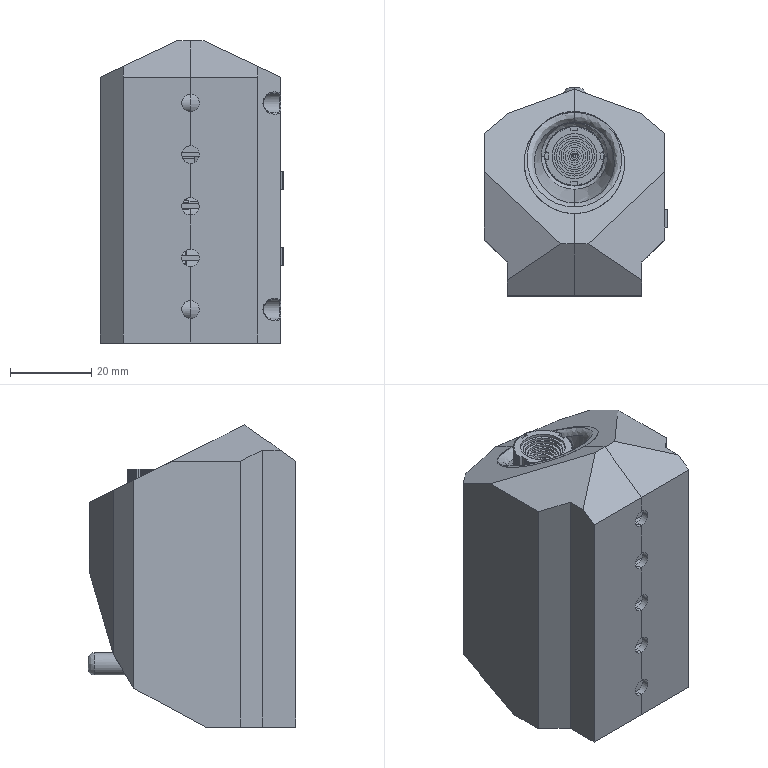Part | SolidWorks | features BaseBody 6 | 6 solids | 1372 faces | box 45.232 x 51.14 x 74.295 mm | volume 38659 mm3 | plane 756 | spline 328 | cylinder 282 | cone 6 | commonest cylinder face diameters 0.4 x86 0.1 x84 4.318 x30 4.9 x12 2.3 x6 2.7 x6